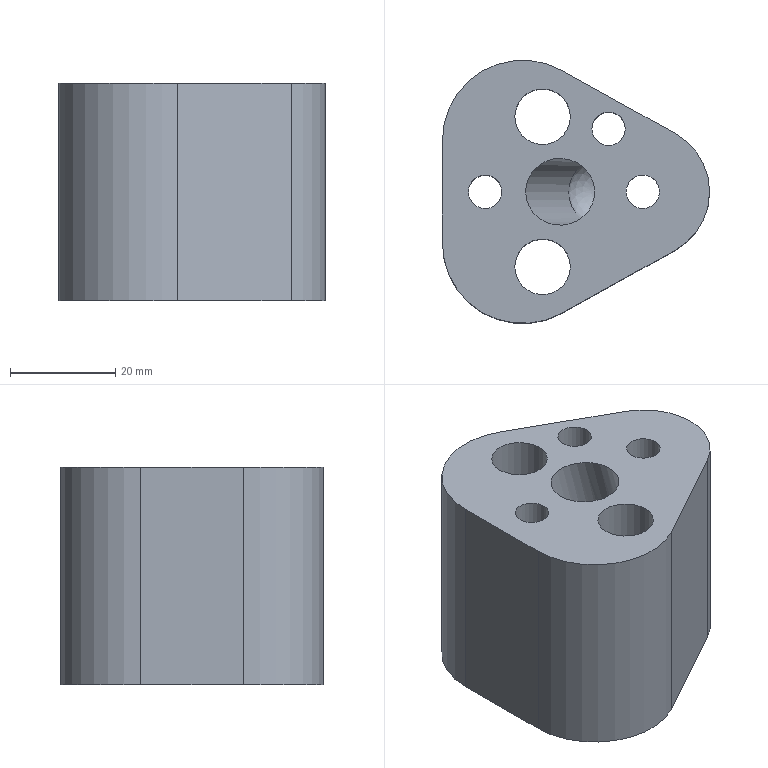Part | STEP file | 1_id486_x_t | 1 solid | 21 faces | box 50.8 x 50.038 x 41.275 mm | volume 56529 mm3 | cylinder 12 | plane 8 | sphere 1 | commonest cylinder face diameters 6.35 x3 10.566 x2 12.7 x2 15.469 x2 30.48 x2 25.4 x1